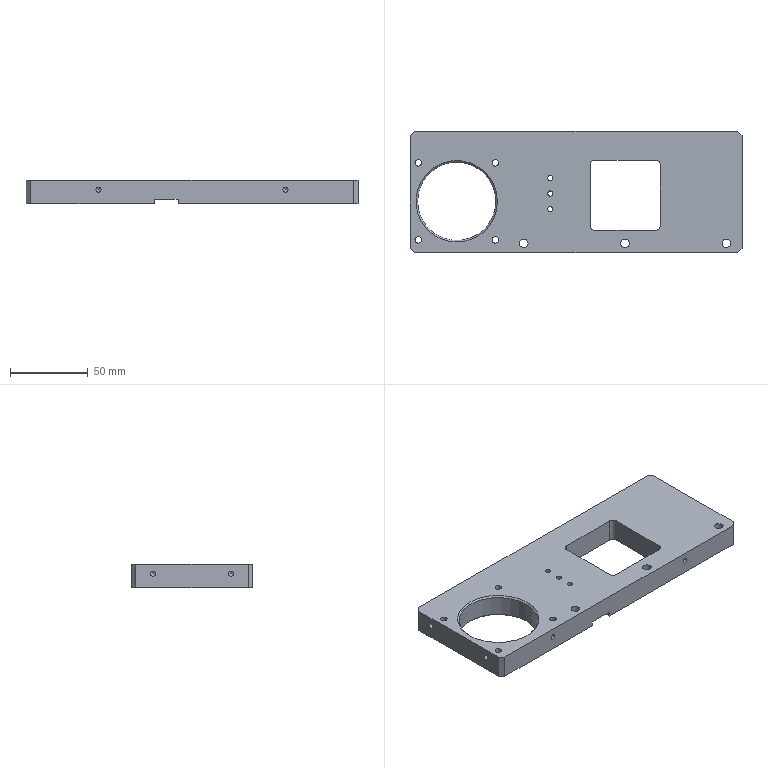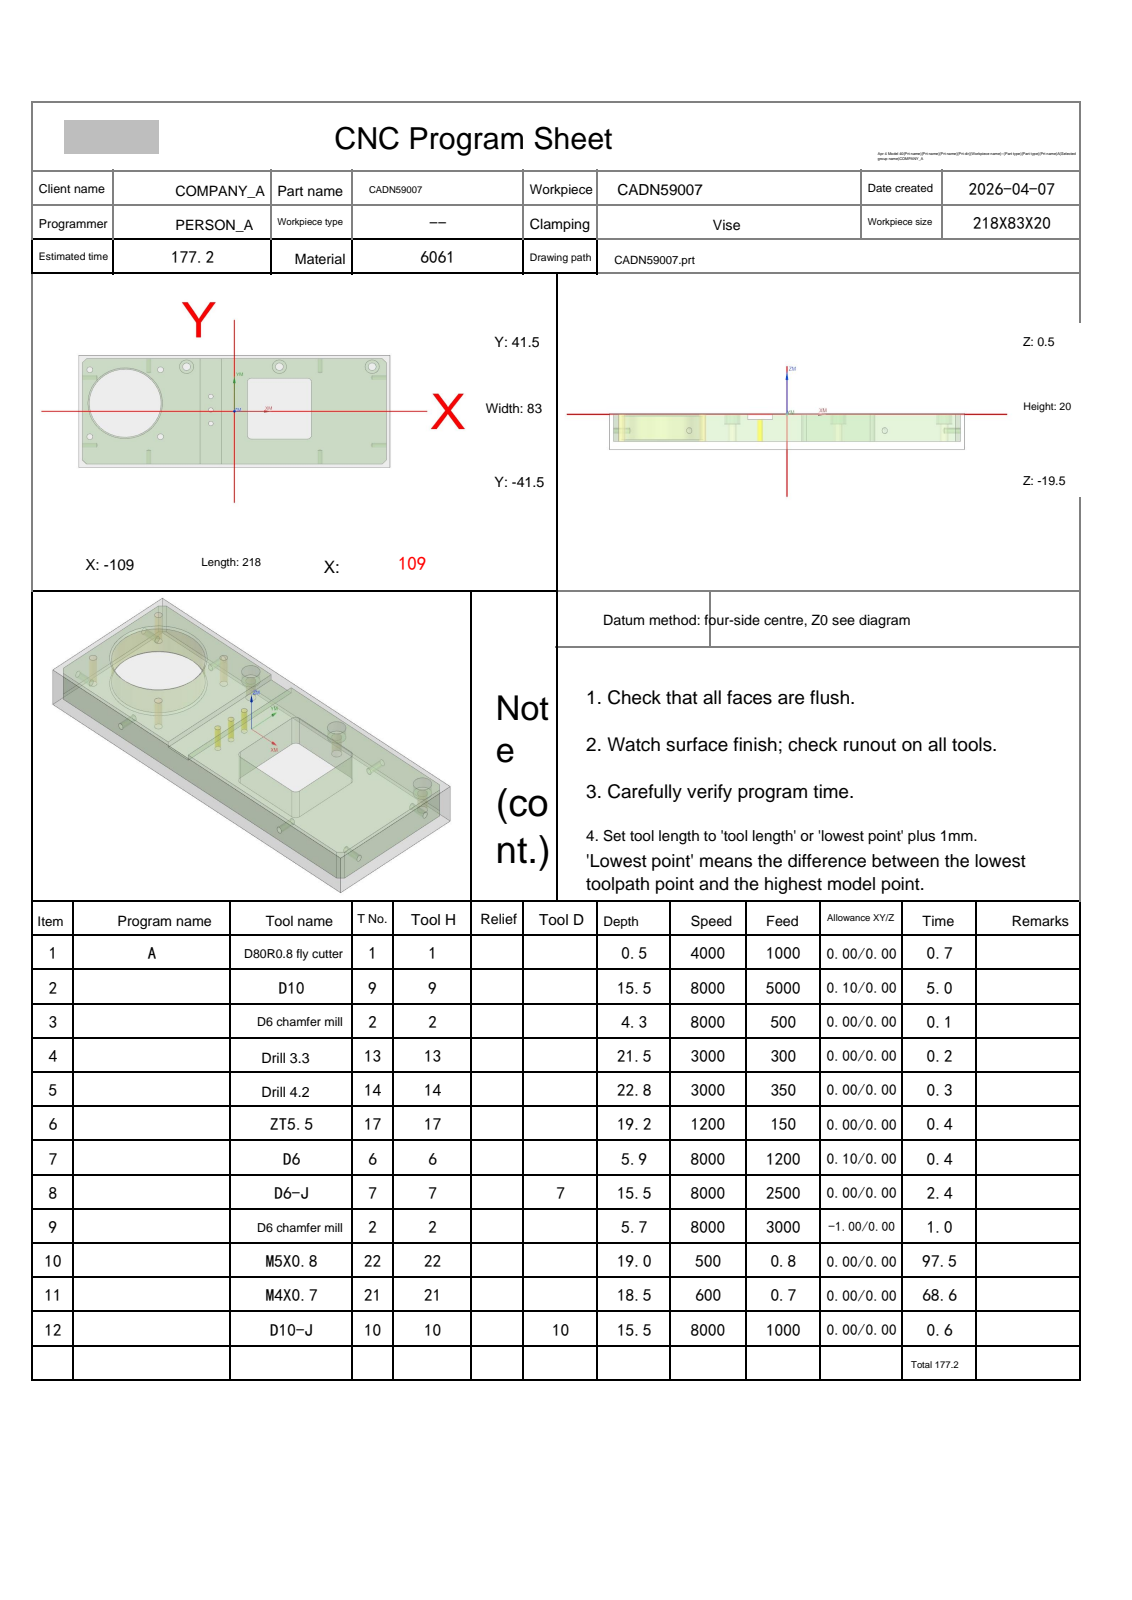NC program | NX | posted by the shop | part box 213 x 78 x 15 mm
Lines 891 to 1965 of 7501:
N8 T07 M06
(D6-J  D=6. R=0. H=07 ce=0.00 di=0.00)
G00 G90 G54 X31.5 Y33. M03 S8000
G43 H07 Z20.
M08
Z0.0
G41 D07
G01 X31.54 Y32.804 F500.
G03 X32.51 Y32.01 I.97 J.196
X33.5 Y33. I0.0 J.99
X33.5 Y33. Z-5. I-2. J0.0
X33.253 Y33.964 Z-5.4 I-2. J0.0
X31.5 Y35. I-1.753 J-.964
X29.5 Y33. I0.0 J-2.
X31.5 Y31. I2. J0.0
X33.5 Y33. I0.0 J2.
X33.253 Y33.964 I-2. J0.0
X32.385 Y34.477 I-.868 J-.477
X31.395 Y33.487 I0.0 J-.99
X31.44 Y33.191 I.99 J0.0
G01 G40 X31.5 Y33.
G00 Z20.
X96.5
Z0.0
G41 D07
G01 X96.54 Y32.804
G03 X97.51 Y32.01 I.97 J.196
X98.5 Y33. I0.0 J.99
X98.5 Y33. Z-5. I-2. J0.0
X98.253 Y33.964 Z-5.4 I-2. J0.0
X96.5 Y35. I-1.753 J-.964
X94.5 Y33. I0.0 J-2.
X96.5 Y31. I2. J0.0
X98.5 Y33. I0.0 J2.
X98.253 Y33.964 I-2. J0.0
X97.385 Y34.477 I-.868 J-.477
X96.395 Y33.487 I0.0 J-.99
X96.44 Y33.191 I.99 J0.0
G01 G40 X96.5 Y33.
G00 Z20.
X-33.5
Z0.0
G41 D07
G01 X-33.46 Y32.804
G03 X-32.49 Y32.01 I.97 J.196
X-31.5 Y33. I0.0 J.99
X-31.5 Y33. Z-5. I-2. J0.0
X-31.747 Y33.964 Z-5.4 I-2. J0.0
X-33.5 Y35. I-1.753 J-.964
X-35.5 Y33. I0.0 J-2.
X-33.5 Y31. I2. J0.0
X-31.5 Y33. I0.0 J2.
X-31.747 Y33.964 I-2. J0.0
X-32.615 Y34.477 I-.868 J-.477
X-33.605 Y33.487 I0.0 J-.99
X-33.56 Y33.191 I.99 J0.0
G01 G40 X-33.5 Y33.
G00 Z20.
G00 G90 X14.816 Y20.6 M03 S6000
Z20.
Z.6
G01 X14.815 Y20.61 Z.471 F2000.
X14.81 Y20.639 Z.355
X14.802 Y20.683 Z.25
X14.79 Y20.741 Z.156
X14.774 Y20.809 Z.072
X14.753 Y20.885 Z-.001
X14.727 Y20.966 Z-.065
X14.696 Y21.05 Z-.12
X14.66 Y21.134 Z-.166
X14.617 Y21.215 Z-.205
X14.568 Y21.291 Z-.236
X14.513 Y21.359 Z-.261
X14.45 Y21.417 Z-.279
X14.38 Y21.461 Z-.291
X14.302 Y21.49 Z-.298
X14.216 Y21.5 Z-.3
X12. F2500.
Y19.284
X12.016 Y19.211 Z-.301
X12.063 Y19.157 Z-.304
X12.136 Y19.119 Z-.308
X12.231 Y19.098 Z-.313
X12.345 Y19.09 Z-.32
X12.474 Y19.096 Z-.328
X12.612 Y19.113 Z-.338
X12.758 Y19.142 Z-.347
X12.906 Y19.179 Z-.358
X13.053 Y19.225 Z-.369
X13.194 Y19.278 Z-.381
X13.431 Y19.39 Z-.404
X13.639 Y19.523 Z-.427
X13.821 Y19.679 Z-.45
X13.977 Y19.861 Z-.473
X14.11 Y20.069 Z-.496
X14.222 Y20.306 Z-.519
X14.275 Y20.447 Z-.531
X14.321 Y20.594 Z-.542
X14.359 Y20.742 Z-.553
X14.387 Y20.888 Z-.562
X14.404 Y21.026 Z-.572
X14.41 Y21.155 Z-.58
X14.402 Y21.269 Z-.587
X14.381 Y21.364 Z-.592
X14.343 Y21.437 Z-.596
X14.289 Y21.484 Z-.599
X14.216 Y21.5 Z-.6
X12.
Y19.284
X12.016 Y19.211 Z-.601
X12.063 Y19.157 Z-.604
X12.136 Y19.119 Z-.608
X12.231 Y19.098 Z-.613
X12.345 Y19.09 Z-.62
X12.474 Y19.096 Z-.628
X12.612 Y19.113 Z-.638
X12.758 Y19.142 Z-.647
X12.906 Y19.179 Z-.658
X13.053 Y19.225 Z-.669
X13.194 Y19.278 Z-.681
X13.431 Y19.39 Z-.704
X13.639 Y19.523 Z-.727
X13.821 Y19.679 Z-.75
X13.977 Y19.861 Z-.773
X14.11 Y20.069 Z-.796
X14.222 Y20.306 Z-.819
X14.275 Y20.447 Z-.831
X14.321 Y20.594 Z-.842
X14.359 Y20.742 Z-.853
X14.387 Y20.888 Z-.862
X14.404 Y21.026 Z-.872
X14.41 Y21.155 Z-.88
X14.402 Y21.269 Z-.887
X14.381 Y21.364 Z-.892
X14.343 Y21.437 Z-.896
X14.289 Y21.484 Z-.899
X14.216 Y21.5 Z-.9
X12.
Y19.284
X12.016 Y19.211 Z-.901
X12.063 Y19.157 Z-.904
X12.136 Y19.119 Z-.908
X12.231 Y19.098 Z-.913
X12.345 Y19.09 Z-.92
X12.474 Y19.096 Z-.928
X12.612 Y19.113 Z-.938
X12.758 Y19.142 Z-.947
X12.906 Y19.179 Z-.958
X13.053 Y19.225 Z-.969
X13.194 Y19.278 Z-.981
X13.431 Y19.39 Z-1.004
X13.639 Y19.523 Z-1.027
X13.821 Y19.679 Z-1.05
X13.977 Y19.861 Z-1.073
X14.11 Y20.069 Z-1.096
X14.222 Y20.306 Z-1.119
X14.275 Y20.447 Z-1.131
X14.321 Y20.594 Z-1.142
X14.359 Y20.742 Z-1.153
X14.387 Y20.888 Z-1.162
X14.404 Y21.026 Z-1.172
X14.41 Y21.155 Z-1.18
X14.402 Y21.269 Z-1.187
X14.381 Y21.364 Z-1.192
X14.343 Y21.437 Z-1.196
X14.289 Y21.484 Z-1.199
X14.216 Y21.5 Z-1.2
X12.
Y19.284
X12.016 Y19.211 Z-1.201
X12.063 Y19.157 Z-1.204
X12.136 Y19.119 Z-1.208
X12.231 Y19.098 Z-1.213
X12.345 Y19.09 Z-1.22
X12.474 Y19.096 Z-1.228
X12.612 Y19.113 Z-1.238
X12.758 Y19.142 Z-1.247
X12.906 Y19.179 Z-1.258
X13.053 Y19.225 Z-1.269
X13.194 Y19.278 Z-1.281
X13.431 Y19.39 Z-1.304
X13.639 Y19.523 Z-1.327
X13.821 Y19.679 Z-1.35
X13.977 Y19.861 Z-1.373
X14.11 Y20.069 Z-1.396
X14.222 Y20.306 Z-1.419
X14.275 Y20.447 Z-1.431
X14.321 Y20.594 Z-1.442
X14.359 Y20.742 Z-1.453
X14.387 Y20.888 Z-1.462
X14.404 Y21.026 Z-1.472
X14.41 Y21.155 Z-1.48
X14.402 Y21.269 Z-1.487
X14.381 Y21.364 Z-1.492
X14.343 Y21.437 Z-1.496
X14.289 Y21.484 Z-1.499
X14.216 Y21.5 Z-1.5
X12.
Y19.284
X12.016 Y19.211 Z-1.501
X12.063 Y19.157 Z-1.504
X12.136 Y19.119 Z-1.508
X12.231 Y19.098 Z-1.513
X12.345 Y19.09 Z-1.52
X12.474 Y19.096 Z-1.528
X12.612 Y19.113 Z-1.538
X12.758 Y19.142 Z-1.547
X12.906 Y19.179 Z-1.558
X13.053 Y19.225 Z-1.569
X13.194 Y19.278 Z-1.581
X13.431 Y19.39 Z-1.604
X13.639 Y19.523 Z-1.627
X13.821 Y19.679 Z-1.65
X13.977 Y19.861 Z-1.673
X14.11 Y20.069 Z-1.696
X14.222 Y20.306 Z-1.719
X14.275 Y20.447 Z-1.731
X14.321 Y20.594 Z-1.742
X14.359 Y20.742 Z-1.753
X14.387 Y20.888 Z-1.762
X14.404 Y21.026 Z-1.772
X14.41 Y21.155 Z-1.78
X14.402 Y21.269 Z-1.787
X14.381 Y21.364 Z-1.792
X14.343 Y21.437 Z-1.796
X14.289 Y21.484 Z-1.799
X14.216 Y21.5 Z-1.8
X12.
Y19.284
X12.016 Y19.211 Z-1.801
X12.063 Y19.157 Z-1.804
X12.136 Y19.119 Z-1.808
X12.231 Y19.098 Z-1.813
X12.345 Y19.09 Z-1.82
X12.474 Y19.096 Z-1.828
X12.612 Y19.113 Z-1.838
X12.758 Y19.142 Z-1.847
X12.906 Y19.179 Z-1.858
X13.053 Y19.225 Z-1.869
X13.194 Y19.278 Z-1.881
X13.431 Y19.39 Z-1.904
X13.639 Y19.523 Z-1.927
X13.821 Y19.679 Z-1.95
X13.977 Y19.861 Z-1.973
X14.11 Y20.069 Z-1.996
X14.222 Y20.306 Z-2.019
X14.275 Y20.447 Z-2.031
X14.321 Y20.594 Z-2.042
X14.359 Y20.742 Z-2.053
X14.387 Y20.888 Z-2.062
X14.404 Y21.026 Z-2.072
X14.41 Y21.155 Z-2.08
X14.402 Y21.269 Z-2.087
X14.381 Y21.364 Z-2.092
X14.343 Y21.437 Z-2.096
X14.289 Y21.484 Z-2.099
X14.216 Y21.5 Z-2.1
X12.
Y19.284
X12.016 Y19.211 Z-2.101
X12.063 Y19.157 Z-2.104
X12.136 Y19.119 Z-2.108
X12.231 Y19.098 Z-2.113
X12.345 Y19.09 Z-2.12
X12.474 Y19.096 Z-2.128
X12.612 Y19.113 Z-2.138
X12.758 Y19.142 Z-2.147
X12.906 Y19.179 Z-2.158
X13.053 Y19.225 Z-2.169
X13.194 Y19.278 Z-2.181
X13.431 Y19.39 Z-2.204
X13.639 Y19.523 Z-2.227
X13.821 Y19.679 Z-2.25
X13.977 Y19.861 Z-2.273
X14.11 Y20.069 Z-2.296
X14.222 Y20.306 Z-2.319
X14.275 Y20.447 Z-2.331
X14.321 Y20.594 Z-2.342
X14.359 Y20.742 Z-2.353
X14.387 Y20.888 Z-2.362
X14.404 Y21.026 Z-2.372
X14.41 Y21.155 Z-2.38
X14.402 Y21.269 Z-2.387
X14.381 Y21.364 Z-2.392
X14.343 Y21.437 Z-2.396
X14.289 Y21.484 Z-2.399
X14.216 Y21.5 Z-2.4
X12.
Y19.284
X12.016 Y19.211 Z-2.401
X12.063 Y19.157 Z-2.404
X12.136 Y19.119 Z-2.408
X12.231 Y19.098 Z-2.413
X12.345 Y19.09 Z-2.42
X12.474 Y19.096 Z-2.428
X12.612 Y19.113 Z-2.438
X12.758 Y19.142 Z-2.447
X12.906 Y19.179 Z-2.458
X13.053 Y19.225 Z-2.469
X13.194 Y19.278 Z-2.481
X13.431 Y19.39 Z-2.504
X13.639 Y19.523 Z-2.527
X13.821 Y19.679 Z-2.55
X13.977 Y19.861 Z-2.573
X14.11 Y20.069 Z-2.596
X14.222 Y20.306 Z-2.619
X14.275 Y20.447 Z-2.631
X14.321 Y20.594 Z-2.642
X14.359 Y20.742 Z-2.653
X14.387 Y20.888 Z-2.662
X14.404 Y21.026 Z-2.672
X14.41 Y21.155 Z-2.68
X14.402 Y21.269 Z-2.687
X14.381 Y21.364 Z-2.692
X14.343 Y21.437 Z-2.696
X14.289 Y21.484 Z-2.699
X14.216 Y21.5 Z-2.7
X12.
Y19.284
X12.016 Y19.211 Z-2.701
X12.063 Y19.157 Z-2.704
X12.136 Y19.119 Z-2.708
X12.231 Y19.098 Z-2.713
X12.345 Y19.09 Z-2.72
X12.474 Y19.096 Z-2.728
X12.612 Y19.113 Z-2.738
X12.758 Y19.142 Z-2.747
X12.906 Y19.179 Z-2.758
X13.053 Y19.225 Z-2.769
X13.194 Y19.278 Z-2.781
X13.431 Y19.39 Z-2.804
X13.639 Y19.523 Z-2.827
X13.821 Y19.679 Z-2.85
X13.977 Y19.861 Z-2.873
X14.11 Y20.069 Z-2.896
X14.222 Y20.306 Z-2.919
X14.275 Y20.447 Z-2.931
X14.321 Y20.594 Z-2.942
X14.359 Y20.742 Z-2.953
X14.387 Y20.888 Z-2.962
X14.404 Y21.026 Z-2.972
X14.41 Y21.155 Z-2.98
X14.402 Y21.269 Z-2.987
X14.381 Y21.364 Z-2.992
X14.343 Y21.437 Z-2.996
X14.289 Y21.484 Z-2.999
X14.216 Y21.5 Z-3.
X12.
Y19.284
X12.016 Y19.211 Z-3.001
X12.063 Y19.157 Z-3.004
X12.136 Y19.119 Z-3.008
X12.231 Y19.098 Z-3.013
X12.345 Y19.09 Z-3.02
X12.474 Y19.096 Z-3.028
X12.612 Y19.113 Z-3.038
X12.758 Y19.142 Z-3.047
X12.906 Y19.179 Z-3.058
X13.053 Y19.225 Z-3.069
X13.194 Y19.278 Z-3.081
X13.431 Y19.39 Z-3.104
X13.639 Y19.523 Z-3.127
X13.821 Y19.679 Z-3.15
X13.977 Y19.861 Z-3.173
X14.11 Y20.069 Z-3.196
X14.222 Y20.306 Z-3.219
X14.275 Y20.447 Z-3.231
X14.321 Y20.594 Z-3.242
X14.359 Y20.742 Z-3.253
X14.387 Y20.888 Z-3.262
X14.404 Y21.026 Z-3.272
X14.41 Y21.155 Z-3.28
X14.402 Y21.269 Z-3.287
X14.381 Y21.364 Z-3.292
X14.343 Y21.437 Z-3.296
X14.289 Y21.484 Z-3.299
X14.216 Y21.5 Z-3.3
X12.
Y19.284
X12.016 Y19.211 Z-3.301
X12.063 Y19.157 Z-3.304
X12.136 Y19.119 Z-3.308
X12.231 Y19.098 Z-3.313
X12.345 Y19.09 Z-3.32
X12.474 Y19.096 Z-3.328
X12.612 Y19.113 Z-3.338
X12.758 Y19.142 Z-3.347
X12.906 Y19.179 Z-3.358
X13.053 Y19.225 Z-3.369
X13.194 Y19.278 Z-3.381
X13.431 Y19.39 Z-3.404
X13.639 Y19.523 Z-3.427
X13.821 Y19.679 Z-3.45
X13.977 Y19.861 Z-3.473
X14.11 Y20.069 Z-3.496
X14.222 Y20.306 Z-3.519
X14.275 Y20.447 Z-3.531
X14.321 Y20.594 Z-3.542
X14.359 Y20.742 Z-3.553
X14.387 Y20.888 Z-3.562
X14.404 Y21.026 Z-3.572
X14.41 Y21.155 Z-3.58
X14.402 Y21.269 Z-3.587
X14.381 Y21.364 Z-3.592
X14.343 Y21.437 Z-3.596
X14.289 Y21.484 Z-3.599
X14.216 Y21.5 Z-3.6
X12.
Y19.284
X12.016 Y19.211 Z-3.601
X12.063 Y19.157 Z-3.604
X12.136 Y19.119 Z-3.608
X12.231 Y19.098 Z-3.613
X12.345 Y19.09 Z-3.62
X12.474 Y19.096 Z-3.628
X12.612 Y19.113 Z-3.638
X12.758 Y19.142 Z-3.647
X12.906 Y19.179 Z-3.658
X13.053 Y19.225 Z-3.669
X13.194 Y19.278 Z-3.681
X13.431 Y19.39 Z-3.704
X13.639 Y19.523 Z-3.727
X13.821 Y19.679 Z-3.75
X13.977 Y19.861 Z-3.773
X14.11 Y20.069 Z-3.796
X14.222 Y20.306 Z-3.819
X14.275 Y20.447 Z-3.831
X14.321 Y20.594 Z-3.842
X14.359 Y20.742 Z-3.853
X14.387 Y20.888 Z-3.862
X14.404 Y21.026 Z-3.872
X14.41 Y21.155 Z-3.88
X14.402 Y21.269 Z-3.887
X14.381 Y21.364 Z-3.892
X14.343 Y21.437 Z-3.896
X14.289 Y21.484 Z-3.899
X14.216 Y21.5 Z-3.9
X12.
Y19.284
X12.016 Y19.211 Z-3.901
X12.063 Y19.157 Z-3.904
X12.136 Y19.119 Z-3.908
X12.231 Y19.098 Z-3.913
X12.345 Y19.09 Z-3.92
X12.474 Y19.096 Z-3.928
X12.612 Y19.113 Z-3.938
X12.758 Y19.142 Z-3.947
X12.906 Y19.179 Z-3.958
X13.053 Y19.225 Z-3.969
X13.194 Y19.278 Z-3.981
X13.431 Y19.39 Z-4.004
X13.639 Y19.523 Z-4.027
X13.821 Y19.679 Z-4.05
X13.977 Y19.861 Z-4.073
X14.11 Y20.069 Z-4.096
X14.222 Y20.306 Z-4.119
X14.275 Y20.447 Z-4.131
X14.321 Y20.594 Z-4.142
X14.359 Y20.742 Z-4.153
X14.387 Y20.888 Z-4.162
X14.404 Y21.026 Z-4.172
X14.41 Y21.155 Z-4.18
X14.402 Y21.269 Z-4.187
X14.381 Y21.364 Z-4.192
X14.343 Y21.437 Z-4.196
X14.289 Y21.484 Z-4.199
X14.216 Y21.5 Z-4.2
X12.
Y19.284
X12.016 Y19.211 Z-4.201
X12.063 Y19.157 Z-4.204
X12.136 Y19.119 Z-4.208
X12.231 Y19.098 Z-4.213
X12.345 Y19.09 Z-4.22
X12.474 Y19.096 Z-4.228
X12.612 Y19.113 Z-4.238
X12.758 Y19.142 Z-4.247
X12.906 Y19.179 Z-4.258
X13.053 Y19.225 Z-4.269
X13.194 Y19.278 Z-4.281
X13.431 Y19.39 Z-4.304
X13.639 Y19.523 Z-4.327
X13.821 Y19.679 Z-4.35
X13.977 Y19.861 Z-4.373
X14.11 Y20.069 Z-4.396
X14.222 Y20.306 Z-4.419
X14.275 Y20.447 Z-4.431
X14.321 Y20.594 Z-4.442
X14.359 Y20.742 Z-4.453
X14.387 Y20.888 Z-4.462
X14.404 Y21.026 Z-4.472
X14.41 Y21.155 Z-4.48
X14.402 Y21.269 Z-4.487
X14.381 Y21.364 Z-4.492
X14.343 Y21.437 Z-4.496
X14.289 Y21.484 Z-4.499
X14.216 Y21.5 Z-4.5
X12.
Y19.284
X12.016 Y19.211 Z-4.501
X12.063 Y19.157 Z-4.504
X12.136 Y19.119 Z-4.508
X12.231 Y19.098 Z-4.513
X12.345 Y19.09 Z-4.52
X12.474 Y19.096 Z-4.528
X12.612 Y19.113 Z-4.538
X12.758 Y19.142 Z-4.547
X12.906 Y19.179 Z-4.558
X13.053 Y19.225 Z-4.569
X13.194 Y19.278 Z-4.581
X13.431 Y19.39 Z-4.604
X13.639 Y19.523 Z-4.627
X13.821 Y19.679 Z-4.65
X13.977 Y19.861 Z-4.673
X14.11 Y20.069 Z-4.696
X14.222 Y20.306 Z-4.719
X14.275 Y20.447 Z-4.731
X14.321 Y20.594 Z-4.742
X14.359 Y20.742 Z-4.753
X14.387 Y20.888 Z-4.762
X14.404 Y21.026 Z-4.772
X14.41 Y21.155 Z-4.78
X14.402 Y21.269 Z-4.787
X14.381 Y21.364 Z-4.792
X14.343 Y21.437 Z-4.796
X14.289 Y21.484 Z-4.799
X14.216 Y21.5 Z-4.8
X12.
Y19.284
X12.016 Y19.211 Z-4.801
X12.063 Y19.157 Z-4.804
X12.136 Y19.119 Z-4.808
X12.231 Y19.098 Z-4.813
X12.345 Y19.09 Z-4.82
X12.474 Y19.096 Z-4.828
X12.612 Y19.113 Z-4.838
X12.758 Y19.142 Z-4.847
X12.906 Y19.179 Z-4.858
X13.053 Y19.225 Z-4.869
X13.194 Y19.278 Z-4.881
X13.431 Y19.39 Z-4.904
X13.639 Y19.523 Z-4.927
X13.821 Y19.679 Z-4.95
X13.977 Y19.861 Z-4.973
X14.11 Y20.069 Z-4.996
X14.222 Y20.306 Z-5.019
X14.275 Y20.447 Z-5.031
X14.321 Y20.594 Z-5.042
X14.359 Y20.742 Z-5.053
X14.387 Y20.888 Z-5.062
X14.404 Y21.026 Z-5.072
X14.41 Y21.155 Z-5.08
X14.402 Y21.269 Z-5.087
X14.381 Y21.364 Z-5.092
X14.343 Y21.437 Z-5.096
X14.289 Y21.484 Z-5.099
X14.216 Y21.5 Z-5.1
X12.
Y19.284
X12.016 Y19.211 Z-5.101
X12.063 Y19.157 Z-5.104
X12.136 Y19.119 Z-5.108
X12.231 Y19.098 Z-5.113
X12.345 Y19.09 Z-5.12
X12.474 Y19.096 Z-5.128
X12.612 Y19.113 Z-5.138
X12.758 Y19.142 Z-5.147
X12.906 Y19.179 Z-5.158
X13.053 Y19.225 Z-5.169
X13.194 Y19.278 Z-5.181
X13.431 Y19.39 Z-5.204
X13.639 Y19.523 Z-5.227
X13.821 Y19.679 Z-5.25
X13.977 Y19.861 Z-5.273
X14.11 Y20.069 Z-5.296
X14.222 Y20.306 Z-5.319
X14.275 Y20.447 Z-5.331
X14.321 Y20.594 Z-5.342
X14.359 Y20.742 Z-5.353
X14.387 Y20.888 Z-5.362
X14.404 Y21.026 Z-5.372
X14.41 Y21.155 Z-5.38
X14.402 Y21.269 Z-5.387
X14.381 Y21.364 Z-5.392
X14.343 Y21.437 Z-5.396
X14.289 Y21.484 Z-5.399
X14.216 Y21.5 Z-5.4
X12.
Y19.284
X12.016 Y19.211 Z-5.401
X12.063 Y19.157 Z-5.404
X12.136 Y19.119 Z-5.408
X12.231 Y19.098 Z-5.413
X12.345 Y19.09 Z-5.42
X12.474 Y19.096 Z-5.428
X12.612 Y19.113 Z-5.438
X12.758 Y19.142 Z-5.447
X12.906 Y19.179 Z-5.458
X13.053 Y19.225 Z-5.469
X13.194 Y19.278 Z-5.481
X13.431 Y19.39 Z-5.504
X13.639 Y19.523 Z-5.527
X13.821 Y19.679 Z-5.55
X13.977 Y19.861 Z-5.573
X14.11 Y20.069 Z-5.596
X14.222 Y20.306 Z-5.619
X14.275 Y20.447 Z-5.631
X14.321 Y20.594 Z-5.642
X14.359 Y20.742 Z-5.653
X14.387 Y20.888 Z-5.662
X14.404 Y21.026 Z-5.672
X14.41 Y21.155 Z-5.68
X14.402 Y21.269 Z-5.687
X14.381 Y21.364 Z-5.692
X14.343 Y21.437 Z-5.696
X14.289 Y21.484 Z-5.699
X14.216 Y21.5 Z-5.7
X12.
Y19.284
X12.016 Y19.211 Z-5.701
X12.063 Y19.157 Z-5.704
X12.136 Y19.119 Z-5.708
X12.231 Y19.098 Z-5.713
X12.345 Y19.09 Z-5.72
X12.474 Y19.096 Z-5.728
X12.612 Y19.113 Z-5.738
X12.758 Y19.142 Z-5.747
X12.906 Y19.179 Z-5.758
X13.053 Y19.225 Z-5.769
X13.194 Y19.278 Z-5.781
X13.431 Y19.39 Z-5.804
X13.639 Y19.523 Z-5.827
X13.821 Y19.679 Z-5.85
X13.977 Y19.861 Z-5.873
X14.11 Y20.069 Z-5.896
X14.222 Y20.306 Z-5.919
X14.275 Y20.447 Z-5.931
X14.321 Y20.594 Z-5.942
X14.359 Y20.742 Z-5.953
X14.387 Y20.888 Z-5.962
X14.404 Y21.026 Z-5.972
X14.41 Y21.155 Z-5.98
X14.402 Y21.269 Z-5.987
X14.381 Y21.364 Z-5.992
X14.343 Y21.437 Z-5.996
X14.289 Y21.484 Z-5.999
X14.216 Y21.5 Z-6.
X12.
Y19.284
X12.016 Y19.211 Z-6.001
X12.063 Y19.157 Z-6.004
X12.136 Y19.119 Z-6.008
X12.231 Y19.098 Z-6.013
X12.345 Y19.09 Z-6.02
X12.474 Y19.096 Z-6.028
X12.612 Y19.113 Z-6.038
X12.758 Y19.142 Z-6.047
X12.906 Y19.179 Z-6.058
X13.053 Y19.225 Z-6.069
X13.194 Y19.278 Z-6.081
X13.431 Y19.39 Z-6.104
X13.639 Y19.523 Z-6.127
X13.821 Y19.679 Z-6.15
X13.977 Y19.861 Z-6.173
X14.11 Y20.069 Z-6.196
X14.222 Y20.306 Z-6.219
X14.275 Y20.447 Z-6.231
X14.321 Y20.594 Z-6.242
X14.359 Y20.742 Z-6.253
X14.387 Y20.888 Z-6.262
X14.404 Y21.026 Z-6.272
X14.41 Y21.155 Z-6.28
X14.402 Y21.269 Z-6.287
X14.381 Y21.364 Z-6.292
X14.343 Y21.437 Z-6.296
X14.289 Y21.484 Z-6.299
X14.216 Y21.5 Z-6.3
X12.
Y19.284
X12.016 Y19.211 Z-6.301
X12.063 Y19.157 Z-6.304
X12.136 Y19.119 Z-6.308
X12.231 Y19.098 Z-6.313
X12.345 Y19.09 Z-6.32
X12.474 Y19.096 Z-6.328
X12.612 Y19.113 Z-6.338
X12.758 Y19.142 Z-6.347
X12.906 Y19.179 Z-6.358
X13.053 Y19.225 Z-6.369
X13.194 Y19.278 Z-6.381
X13.431 Y19.39 Z-6.404
X13.639 Y19.523 Z-6.427
X13.821 Y19.679 Z-6.45
X13.977 Y19.861 Z-6.473
X14.11 Y20.069 Z-6.496
X14.222 Y20.306 Z-6.519
X14.275 Y20.447 Z-6.531
X14.321 Y20.594 Z-6.542
X14.359 Y20.742 Z-6.553
X14.387 Y20.888 Z-6.562
X14.404 Y21.026 Z-6.572
X14.41 Y21.155 Z-6.58
X14.402 Y21.269 Z-6.587
X14.381 Y21.364 Z-6.592
X14.343 Y21.437 Z-6.596
X14.289 Y21.484 Z-6.599
X14.216 Y21.5 Z-6.6
X12.
Y19.284
X12.016 Y19.211 Z-6.601
X12.063 Y19.157 Z-6.604
X12.136 Y19.119 Z-6.608
X12.231 Y19.098 Z-6.613
X12.345 Y19.09 Z-6.62
X12.474 Y19.096 Z-6.628
X12.612 Y19.113 Z-6.638
X12.758 Y19.142 Z-6.647
X12.906 Y19.179 Z-6.658
X13.053 Y19.225 Z-6.669
X13.194 Y19.278 Z-6.681
X13.431 Y19.39 Z-6.704
X13.639 Y19.523 Z-6.727
X13.821 Y19.679 Z-6.75
X13.977 Y19.861 Z-6.773
X14.11 Y20.069 Z-6.796
X14.222 Y20.306 Z-6.819
X14.275 Y20.447 Z-6.831
X14.321 Y20.594 Z-6.842
X14.359 Y20.742 Z-6.853
X14.387 Y20.888 Z-6.862
X14.404 Y21.026 Z-6.872
X14.41 Y21.155 Z-6.88
X14.402 Y21.269 Z-6.887
X14.381 Y21.364 Z-6.892
X14.343 Y21.437 Z-6.896
X14.289 Y21.484 Z-6.899
X14.216 Y21.5 Z-6.9
X12.
Y19.284
X12.016 Y19.211 Z-6.901
X12.063 Y19.157 Z-6.904
X12.136 Y19.119 Z-6.908
X12.231 Y19.098 Z-6.913
X12.345 Y19.09 Z-6.92
X12.474 Y19.096 Z-6.928
X12.612 Y19.113 Z-6.938
X12.758 Y19.142 Z-6.947
X12.906 Y19.179 Z-6.958
X13.053 Y19.225 Z-6.969
X13.194 Y19.278 Z-6.981
X13.431 Y19.39 Z-7.004
X13.639 Y19.523 Z-7.027
X13.821 Y19.679 Z-7.05
X13.977 Y19.861 Z-7.073
X14.11 Y20.069 Z-7.096
X14.222 Y20.306 Z-7.119
X14.275 Y20.447 Z-7.131
X14.321 Y20.594 Z-7.142
X14.359 Y20.742 Z-7.153
X14.387 Y20.888 Z-7.162
X14.404 Y21.026 Z-7.172
X14.41 Y21.155 Z-7.18
X14.402 Y21.269 Z-7.187
X14.381 Y21.364 Z-7.192
X14.343 Y21.437 Z-7.196
X14.289 Y21.484 Z-7.199
X14.216 Y21.5 Z-7.2
X12.
Y19.284
X12.016 Y19.211 Z-7.201
X12.063 Y19.157 Z-7.204
X12.136 Y19.119 Z-7.208
X12.231 Y19.098 Z-7.213
X12.345 Y19.09 Z-7.22
X12.474 Y19.096 Z-7.228
X12.612 Y19.113 Z-7.238
X12.758 Y19.142 Z-7.247
X12.906 Y19.179 Z-7.258
X13.053 Y19.225 Z-7.269
X13.194 Y19.278 Z-7.281
X13.431 Y19.39 Z-7.304
X13.639 Y19.523 Z-7.327
X13.821 Y19.679 Z-7.35
X13.977 Y19.861 Z-7.373
X14.11 Y20.069 Z-7.396
X14.222 Y20.306 Z-7.419
X14.275 Y20.447 Z-7.431
X14.321 Y20.594 Z-7.442
X14.359 Y20.742 Z-7.453
X14.387 Y20.888 Z-7.462
X14.404 Y21.026 Z-7.472
X14.41 Y21.155 Z-7.48
X14.402 Y21.269 Z-7.487
X14.381 Y21.364 Z-7.492
X14.343 Y21.437 Z-7.496
X14.289 Y21.484 Z-7.499
X14.216 Y21.5 Z-7.5
X12.
Y19.284
X12.016 Y19.211 Z-7.501
X12.063 Y19.157 Z-7.504
X12.136 Y19.119 Z-7.508
X12.231 Y19.098 Z-7.513
X12.345 Y19.09 Z-7.52
X12.474 Y19.096 Z-7.528
X12.612 Y19.113 Z-7.538
X12.758 Y19.142 Z-7.547
X12.906 Y19.179 Z-7.558
X13.053 Y19.225 Z-7.569
X13.194 Y19.278 Z-7.581
X13.431 Y19.39 Z-7.604
X13.639 Y19.523 Z-7.627
X13.821 Y19.679 Z-7.65
X13.977 Y19.861 Z-7.673
X14.11 Y20.069 Z-7.696
X14.222 Y20.306 Z-7.719
X14.275 Y20.447 Z-7.731
X14.321 Y20.594 Z-7.742
X14.359 Y20.742 Z-7.753
X14.387 Y20.888 Z-7.762
X14.404 Y21.026 Z-7.772
X14.41 Y21.155 Z-7.78
X14.402 Y21.269 Z-7.787
X14.381 Y21.364 Z-7.792
X14.343 Y21.437 Z-7.796
X14.289 Y21.484 Z-7.799
X14.216 Y21.5 Z-7.8
X12.
Y19.284
X12.016 Y19.211 Z-7.801
X12.063 Y19.157 Z-7.804
X12.136 Y19.119 Z-7.808
X12.231 Y19.098 Z-7.813
X12.345 Y19.09 Z-7.82
X12.474 Y19.096 Z-7.828
X12.612 Y19.113 Z-7.838
X12.758 Y19.142 Z-7.847
X12.906 Y19.179 Z-7.858
X13.053 Y19.225 Z-7.869
X13.194 Y19.278 Z-7.881
X13.431 Y19.39 Z-7.904
X13.639 Y19.523 Z-7.927
X13.821 Y19.679 Z-7.95
X13.977 Y19.861 Z-7.973
X14.11 Y20.069 Z-7.996
X14.222 Y20.306 Z-8.019
X14.275 Y20.447 Z-8.031
X14.321 Y20.594 Z-8.042
X14.359 Y20.742 Z-8.053
X14.387 Y20.888 Z-8.062
X14.404 Y21.026 Z-8.072
X14.41 Y21.155 Z-8.08
X14.402 Y21.269 Z-8.087
X14.381 Y21.364 Z-8.092
X14.343 Y21.437 Z-8.096
X14.289 Y21.484 Z-8.099
X14.216 Y21.5 Z-8.1
X12.
Y19.284
X12.016 Y19.211 Z-8.101
X12.063 Y19.157 Z-8.104
X12.136 Y19.119 Z-8.108
X12.231 Y19.098 Z-8.113
X12.345 Y19.09 Z-8.12
X12.474 Y19.096 Z-8.128
X12.612 Y19.113 Z-8.138
X12.758 Y19.142 Z-8.147
X12.906 Y19.179 Z-8.158
X13.053 Y19.225 Z-8.169
X13.194 Y19.278 Z-8.181
X13.431 Y19.39 Z-8.204
X13.639 Y19.523 Z-8.227
X13.821 Y19.679 Z-8.25
X13.977 Y19.861 Z-8.273
X14.11 Y20.069 Z-8.296
X14.222 Y20.306 Z-8.319
X14.275 Y20.447 Z-8.331
X14.321 Y20.594 Z-8.342
X14.359 Y20.742 Z-8.353
X14.387 Y20.888 Z-8.362
X14.404 Y21.026 Z-8.372
X14.41 Y21.155 Z-8.38
X14.402 Y21.269 Z-8.387
X14.381 Y21.364 Z-8.392
X14.343 Y21.437 Z-8.396
X14.289 Y21.484 Z-8.399
X14.216 Y21.5 Z-8.4
X12.
Y19.284
X12.016 Y19.211 Z-8.401
X12.063 Y19.157 Z-8.404
X12.136 Y19.119 Z-8.408
X12.231 Y19.098 Z-8.413
X12.345 Y19.09 Z-8.42
X12.474 Y19.096 Z-8.428
X12.612 Y19.113 Z-8.438
X12.758 Y19.142 Z-8.447
X12.906 Y19.179 Z-8.458
X13.053 Y19.225 Z-8.469
X13.194 Y19.278 Z-8.481
X13.431 Y19.39 Z-8.504
X13.639 Y19.523 Z-8.527
X13.821 Y19.679 Z-8.55
X13.977 Y19.861 Z-8.573
X14.11 Y20.069 Z-8.596
X14.222 Y20.306 Z-8.619
X14.275 Y20.447 Z-8.631
X14.321 Y20.594 Z-8.642
X14.359 Y20.742 Z-8.653
X14.387 Y20.888 Z-8.662
X14.404 Y21.026 Z-8.672
X14.41 Y21.155 Z-8.68
X14.402 Y21.269 Z-8.687
X14.381 Y21.364 Z-8.692
X14.343 Y21.437 Z-8.696
X14.289 Y21.484 Z-8.699
X14.216 Y21.5 Z-8.7
X12.
Y19.284
X12.016 Y19.211 Z-8.701
X12.063 Y19.157 Z-8.704
X12.136 Y19.119 Z-8.708
X12.231 Y19.098 Z-8.713
X12.345 Y19.09 Z-8.72
X12.474 Y19.096 Z-8.728
X12.612 Y19.113 Z-8.738
X12.758 Y19.142 Z-8.747
X12.906 Y19.179 Z-8.758
X13.053 Y19.225 Z-8.769
X13.194 Y19.278 Z-8.781
X13.431 Y19.39 Z-8.804
X13.639 Y19.523 Z-8.827
X13.821 Y19.679 Z-8.85
X13.977 Y19.861 Z-8.873
X14.11 Y20.069 Z-8.896
X14.222 Y20.306 Z-8.919
X14.275 Y20.447 Z-8.931
X14.321 Y20.594 Z-8.942
X14.359 Y20.742 Z-8.953
X14.387 Y20.888 Z-8.962
X14.404 Y21.026 Z-8.972
X14.41 Y21.155 Z-8.98
X14.402 Y21.269 Z-8.987
X14.381 Y21.364 Z-8.992
X14.343 Y21.437 Z-8.996
X14.289 Y21.484 Z-8.999
X14.216 Y21.5 Z-9.
X12.
Y19.284
X12.016 Y19.211 Z-9.001
X12.063 Y19.157 Z-9.004
X12.136 Y19.119 Z-9.008
X12.231 Y19.098 Z-9.013
X12.345 Y19.09 Z-9.02
X12.474 Y19.096 Z-9.028
X12.612 Y19.113 Z-9.038
X12.758 Y19.142 Z-9.047
X12.906 Y19.179 Z-9.058
X13.053 Y19.225 Z-9.069
X13.194 Y19.278 Z-9.081
X13.431 Y19.39 Z-9.104
X13.639 Y19.523 Z-9.127
X13.821 Y19.679 Z-9.15
X13.977 Y19.861 Z-9.173
X14.11 Y20.069 Z-9.196
X14.222 Y20.306 Z-9.219
X14.275 Y20.447 Z-9.231
X14.321 Y20.594 Z-9.242
X14.359 Y20.742 Z-9.253
X14.387 Y20.888 Z-9.262
X14.404 Y21.026 Z-9.272
X14.41 Y21.155 Z-9.28
X14.402 Y21.269 Z-9.287
X14.381 Y21.364 Z-9.292
X14.343 Y21.437 Z-9.296
X14.289 Y21.484 Z-9.299
X14.216 Y21.5 Z-9.3
X12.
Y19.284
X12.016 Y19.211 Z-9.301
X12.063 Y19.157 Z-9.304
X12.136 Y19.119 Z-9.308
X12.231 Y19.098 Z-9.313
X12.345 Y19.09 Z-9.32
X12.474 Y19.096 Z-9.328
X12.612 Y19.113 Z-9.338
X12.758 Y19.142 Z-9.347
X12.906 Y19.179 Z-9.358
X13.053 Y19.225 Z-9.369
X13.194 Y19.278 Z-9.381
X13.431 Y19.39 Z-9.404
X13.639 Y19.523 Z-9.427
X13.821 Y19.679 Z-9.45
X13.977 Y19.861 Z-9.473
X14.11 Y20.069 Z-9.496
X14.222 Y20.306 Z-9.519
X14.275 Y20.447 Z-9.531
X14.321 Y20.594 Z-9.542
X14.359 Y20.742 Z-9.553
X14.387 Y20.888 Z-9.562
X14.404 Y21.026 Z-9.572
X14.41 Y21.155 Z-9.58
X14.402 Y21.269 Z-9.587
X14.381 Y21.364 Z-9.592
X14.343 Y21.437 Z-9.596
X14.289 Y21.484 Z-9.599
X14.216 Y21.5 Z-9.6
X12.
Y19.284
X12.016 Y19.211 Z-9.601
X12.063 Y19.157 Z-9.604
X12.136 Y19.119 Z-9.608
X12.231 Y19.098 Z-9.613
X12.345 Y19.09 Z-9.62
X12.474 Y19.096 Z-9.628
X12.612 Y19.113 Z-9.638
X12.758 Y19.142 Z-9.647
X12.906 Y19.179 Z-9.658
X13.053 Y19.225 Z-9.669
X13.194 Y19.278 Z-9.681
X13.431 Y19.39 Z-9.704
X13.639 Y19.523 Z-9.727
X13.821 Y19.679 Z-9.75
X13.977 Y19.861 Z-9.773
X14.11 Y20.069 Z-9.796
X14.222 Y20.306 Z-9.819
X14.275 Y20.447 Z-9.831
X14.321 Y20.594 Z-9.842
X14.359 Y20.742 Z-9.853
X14.387 Y20.888 Z-9.862
X14.404 Y21.026 Z-9.872
X14.41 Y21.155 Z-9.88
X14.402 Y21.269 Z-9.887
X14.381 Y21.364 Z-9.892
X14.343 Y21.437 Z-9.896
X14.289 Y21.484 Z-9.899
X14.216 Y21.5 Z-9.9
X12.
Y19.284
X12.016 Y19.211 Z-9.901
X12.063 Y19.157 Z-9.904
X12.136 Y19.119 Z-9.908
X12.231 Y19.098 Z-9.913
X12.345 Y19.09 Z-9.92
X12.474 Y19.096 Z-9.928
X12.612 Y19.113 Z-9.938
X12.758 Y19.142 Z-9.947
X12.906 Y19.179 Z-9.958
X13.053 Y19.225 Z-9.969
X13.194 Y19.278 Z-9.981
X13.431 Y19.39 Z-10.004
X13.639 Y19.523 Z-10.027
X13.821 Y19.679 Z-10.05
X13.977 Y19.861 Z-10.073
X14.11 Y20.069 Z-10.096
X14.222 Y20.306 Z-10.119
X14.275 Y20.447 Z-10.131
X14.321 Y20.594 Z-10.142
X14.359 Y20.742 Z-10.153
X14.387 Y20.888 Z-10.162
X14.404 Y21.026 Z-10.172
X14.41 Y21.155 Z-10.18
X14.402 Y21.269 Z-10.187
X14.381 Y21.364 Z-10.192
X14.343 Y21.437 Z-10.196
X14.289 Y21.484 Z-10.199
X14.216 Y21.5 Z-10.2
X12.
Y19.284
X12.016 Y19.211 Z-10.201
X12.063 Y19.157 Z-10.204
X12.136 Y19.119 Z-10.208
X12.231 Y19.098 Z-10.213
X12.345 Y19.09 Z-10.22
X12.474 Y19.096 Z-10.228